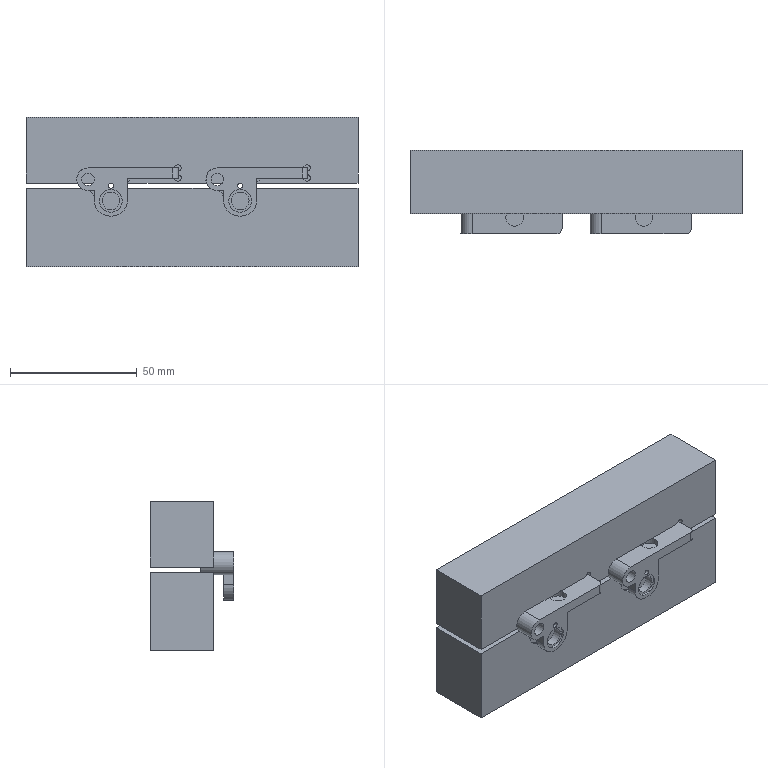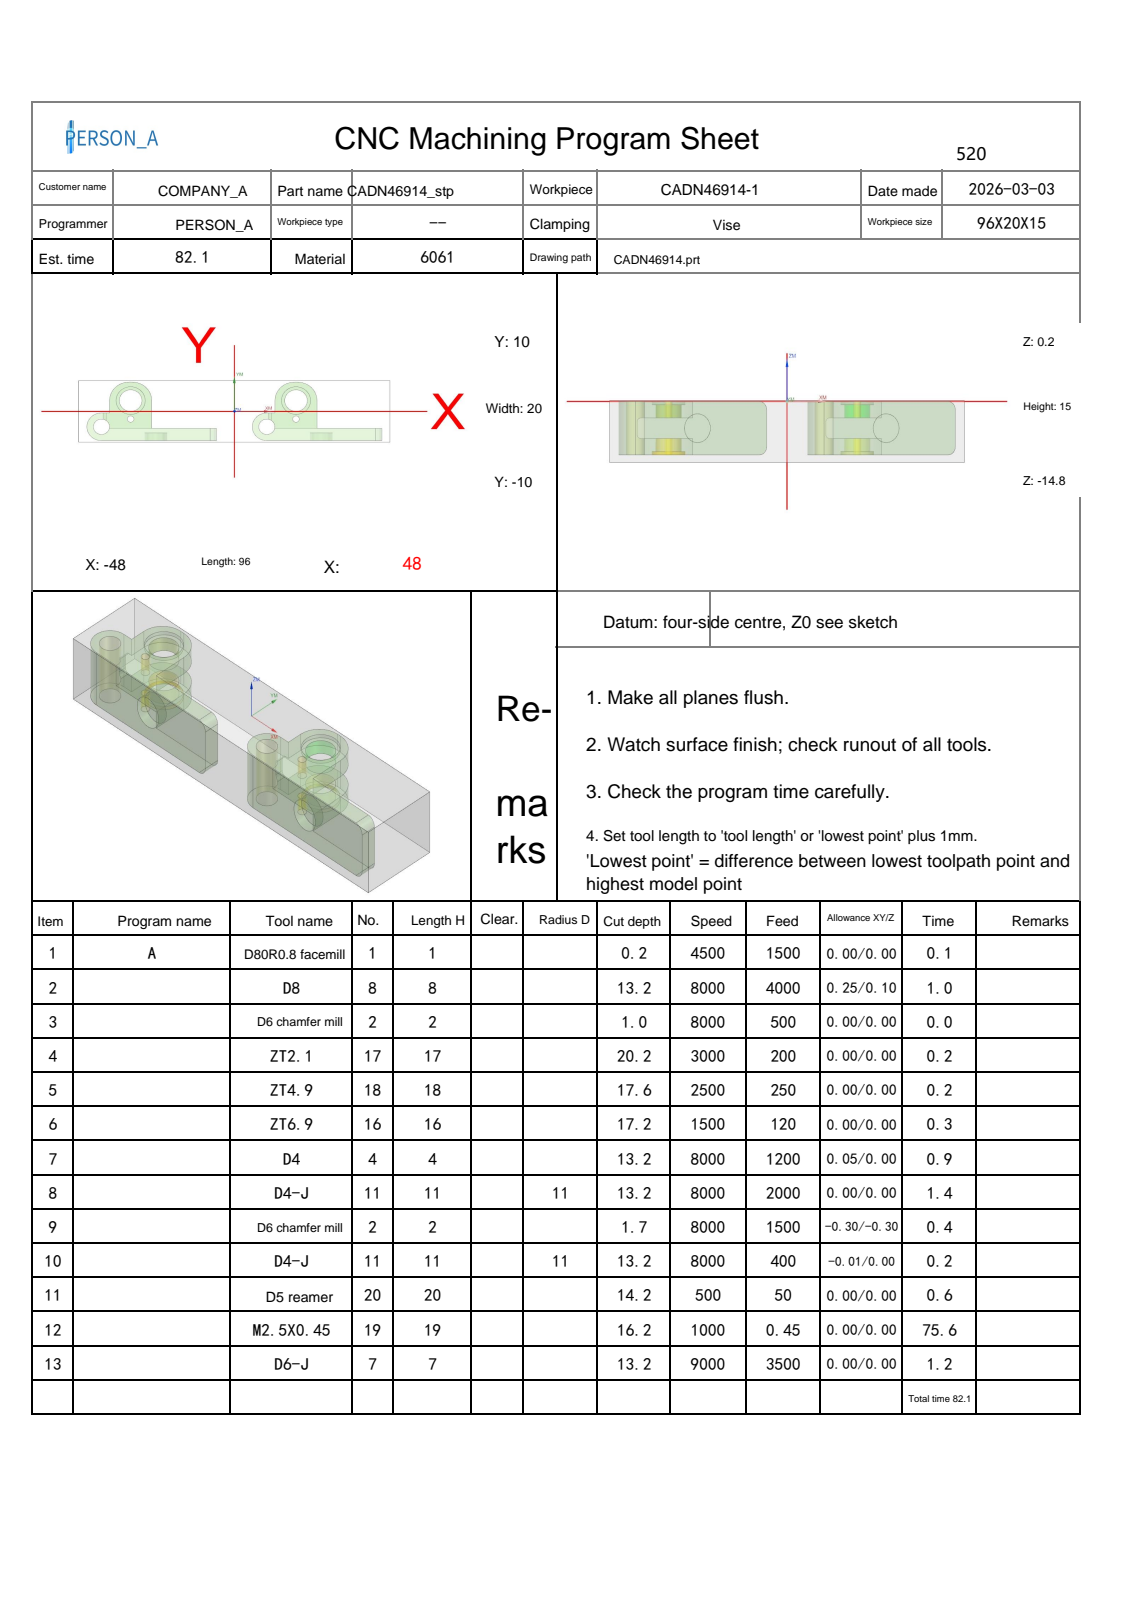NC program | NX | posted by the shop | part box 131 x 33 x 59 mm
Lines 8889 to 9139 of 12027:
N9 T02 M06
(D6 chamfer mill  D=6. R=0. H=02 ce=0.00 di=0.00)
G00 G90 G54 X-32. Y-2.5 M03 S8000
G43 H02 Z50.
M08
G98 G81 X-32. Y-2.5 Z-1.475 R3. F500.
X19.
G80
G00 Z50.
G00 G90 X-41.784 Y-5.157 M03 S8000
Z50.
Z-.5
G01 Z-1. F500.
X-42.5 Y-5.3
G03 X-41. Y-6.8 I1.5 J0.0
X-39.2 Y-5. I0.0 J1.8
X-41. Y-3.2 I-1.8 J0.0
X-42.8 Y-5. I0.0 J-1.8
X-41. Y-6.8 I1.8 J0.0
X-39.5 Y-5.3 I0.0 J1.5
G01 X-40.216 Y-5.157
Z-.5
G00 Z50.
X9.216
Z-.5
G01 Z-1.
X8.5 Y-5.3
G03 X10. Y-6.8 I1.5 J0.0
X11.8 Y-5. I0.0 J1.8
X10. Y-3.2 I-1.8 J0.0
X8.2 Y-5. I0.0 J-1.8
X10. Y-6.8 I1.8 J0.0
X11.5 Y-5.3 I0.0 J1.5
G01 X10.784 Y-5.157
Z-.5
G00 Z50.
G00 G90 X-7.114 Y-10.227 M03 S6500
Z50.
Z.642
G01 Z-.7 F1500.
G03 X-7.4 Y-10.027 I-1.286 J-1.532
G01 X-7.446 Y-9.997
X-7.5 Y-10.
X-41.
G02 X-46. Y-5. I0.0 J5.
X-41. Y0.0 I5. J0.0
G01 X-39.
Y3.5
G02 X-32.5 Y10. I6.5 J0.0
G01 X-31.5
G02 X-25. Y3.5 I0.0 J-6.5
G01 Y-5.
X-7.5
X-7.446 Y-5.003
X-7.4 Y-4.973
G03 X-7.114 Y-4.773 I-1. J1.732
G01 Z.642
G00 Z10.
X-32.4 Y-.299
Z.725
G01 Z-.7
G03 X-32.102 Y-.48 I1.183 J1.613
G01 X-32.054 Y-.506
X-32. Y-.5
G03 X-28. Y3.5 I0.0 J4.
X-32. Y7.5 I-4. J0.0
X-36. Y3.5 I0.0 J-4.
X-32. Y-.5 I4. J0.0
G01 X-31.946 Y-.506
X-31.898 Y-.48
G03 X-31.6 Y-.299 I-.885 J1.794
G01 Z.725
G00 Z3.05
X-41.404 Y-6.808
Z.759
G01 Z-.7
G03 X-41.102 Y-6.982 I1.147 J1.638
G01 X-41.054 Y-7.008
X-41. Y-7.
G03 X-39. Y-5. I0.0 J2.
X-41. Y-3. I-2. J0.0
X-43. Y-5. I0.0 J-2.
X-41.347 Y-6.97 I2. J0.0
G01 X-41. Y-7.
X-40.946 Y-7.008
X-40.898 Y-6.982
G03 X-40.596 Y-6.808 I-.845 J1.813
G01 Z.759
G00 Z10.
X43.886 Y-10.227
Z.642
G01 Z-.7
G03 X43.6 Y-10.027 I-1.286 J-1.532
G01 X43.554 Y-9.997
X43.5 Y-10.
X10.
G02 X5. Y-5. I0.0 J5.
X10. Y0.0 I5. J0.0
G01 X12.
Y3.5
G02 X18.5 Y10. I6.5 J0.0
G01 X19.5
G02 X26. Y3.5 I0.0 J-6.5
G01 Y-5.
X43.5
X43.554 Y-5.003
X43.6 Y-4.973
G03 X43.886 Y-4.773 I-1. J1.732
G01 Z.642
G00 Z10.
X18.6 Y-.299
Z.725
G01 Z-.7
G03 X18.898 Y-.48 I1.183 J1.613
G01 X18.946 Y-.506
X19. Y-.5
G03 X23. Y3.5 I0.0 J4.
X19. Y7.5 I-4. J0.0
X15. Y3.5 I0.0 J-4.
X19. Y-.5 I4. J0.0
G01 X19.054 Y-.506
X19.102 Y-.48
G03 X19.4 Y-.299 I-.885 J1.794
G01 Z.725
G00 Z3.05
X9.596 Y-6.808
Z.759
G01 Z-.7
G03 X9.898 Y-6.982 I1.147 J1.638
G01 X9.946 Y-7.008
X10. Y-7.
G03 X12. Y-5. I0.0 J2.
X10. Y-3. I-2. J0.0
X8. Y-5. I0.0 J-2.
X9.653 Y-6.97 I2. J0.0
G01 X10. Y-7.
X10.054 Y-7.008
X10.102 Y-6.982
G03 X10.404 Y-6.808 I-.845 J1.813
G01 Z.759
G00 Z3.05
X18.599 Y.697
Z-.06
G01 Z-1.5
G03 X18.898 Y.519 I1.167 J1.624
G01 X18.946 Y.493
X19. Y.5
G03 X22. Y3.5 I0.0 J3.
X19. Y6.5 I-3. J0.0
X16. Y3.5 I0.0 J-3.
X19. Y.5 I3. J0.0
G01 X19.054 Y.493
X19.102 Y.519
G03 X19.401 Y.697 I-.868 J1.802
G01 Z-.06
G00 Z10.
X-32.401
Z-.06
G01 Z-1.5
G03 X-32.102 Y.519 I1.167 J1.624
G01 X-32.054 Y.493
X-32. Y.5
G03 X-29. Y3.5 I0.0 J3.
X-32. Y6.5 I-3. J0.0
X-35. Y3.5 I0.0 J-3.
X-32. Y.5 I3. J0.0
G01 X-31.946 Y.493
X-31.898 Y.519
G03 X-31.599 Y.697 I-.868 J1.802
G01 Z-.06
G00 Z50.
G91 G28 Z0.0
M05
M09
G91 G28 Z0.0
M01
N10 T11 M06
(D4-J  D=4. R=0. H=11 ce=-0.01 di=0.00)
G00 G90 G54 X-32. Y3.5 M03 S8000
G43 H11 Z50.
M08
Z-.3
G41 D11
G01 X-31.948 Y3.307 F400.
G03 X-31.232 Y2.758 I.716 J.193
X-30.49 Y3.5 I0.0 J.742
X-30.49 Y3.5 Z-5.3 I-1.51 J0.0
X-30.49 Y3.5 Z-10.3 I-1.51 J0.0
X-33.463 Y3.124 Z-13. I-1.51 J0.0
X-32. Y1.99 I1.463 J.376
X-30.49 Y3.5 I0.0 J1.51
X-32. Y5.01 I-1.51 J0.0
X-33.51 Y3.5 I0.0 J-1.51
X-33.463 Y3.124 I1.51 J0.0
X-32.744 Y2.567 I.718 J.184
X-32.002 Y3.3 I0.0 J.742
G01 G40 X-32. Y3.5
G00 Z50.
X19.
Z-.3
G41 D11
G01 X19.052 Y3.307
G03 X19.768 Y2.758 I.716 J.193
X20.51 Y3.5 I0.0 J.742
X20.51 Y3.5 Z-5.3 I-1.51 J0.0
X20.51 Y3.5 Z-10.3 I-1.51 J0.0
X17.537 Y3.124 Z-13. I-1.51 J0.0
X19. Y1.99 I1.463 J.376
X20.51 Y3.5 I0.0 J1.51
X19. Y5.01 I-1.51 J0.0
X17.49 Y3.5 I0.0 J-1.51
X17.537 Y3.124 I1.51 J0.0
X18.256 Y2.567 I.718 J.184
X18.998 Y3.3 I0.0 J.742
G01 G40 X19. Y3.5
G00 Z50.
G91 G28 Z0.0
M05
M09
G91 G28 Z0.0
M01
N11 T20 M06
(D5 reamer D=5. DR_a=180 H=20)
G00 G90 G54 X-41. Y-5. M03 S500
G43 H20 Z50.
M08
G98 G81 X-41. Y-5. Z-14. R1. F50.
X10.
G80
G00 Z50.
G91 G28 Z0.0
M05
M09
G91 G28 Z0.0
M01
N12 T19 M06
(M2.5X0.45 D=2.05 DR_a=180 H=19)
G00 G90 G54 X-32. Y-2.5 M03 S1000
G43 H19 Z50.
M08
G95
G98 G84 X-32. Y-2.5 Z-16. R1. F.45 Q5.
X19.
G80
G94
G00 Z50.
G91 G28 Z0.0
M05
M09
G91 G28 Z0.0
M01